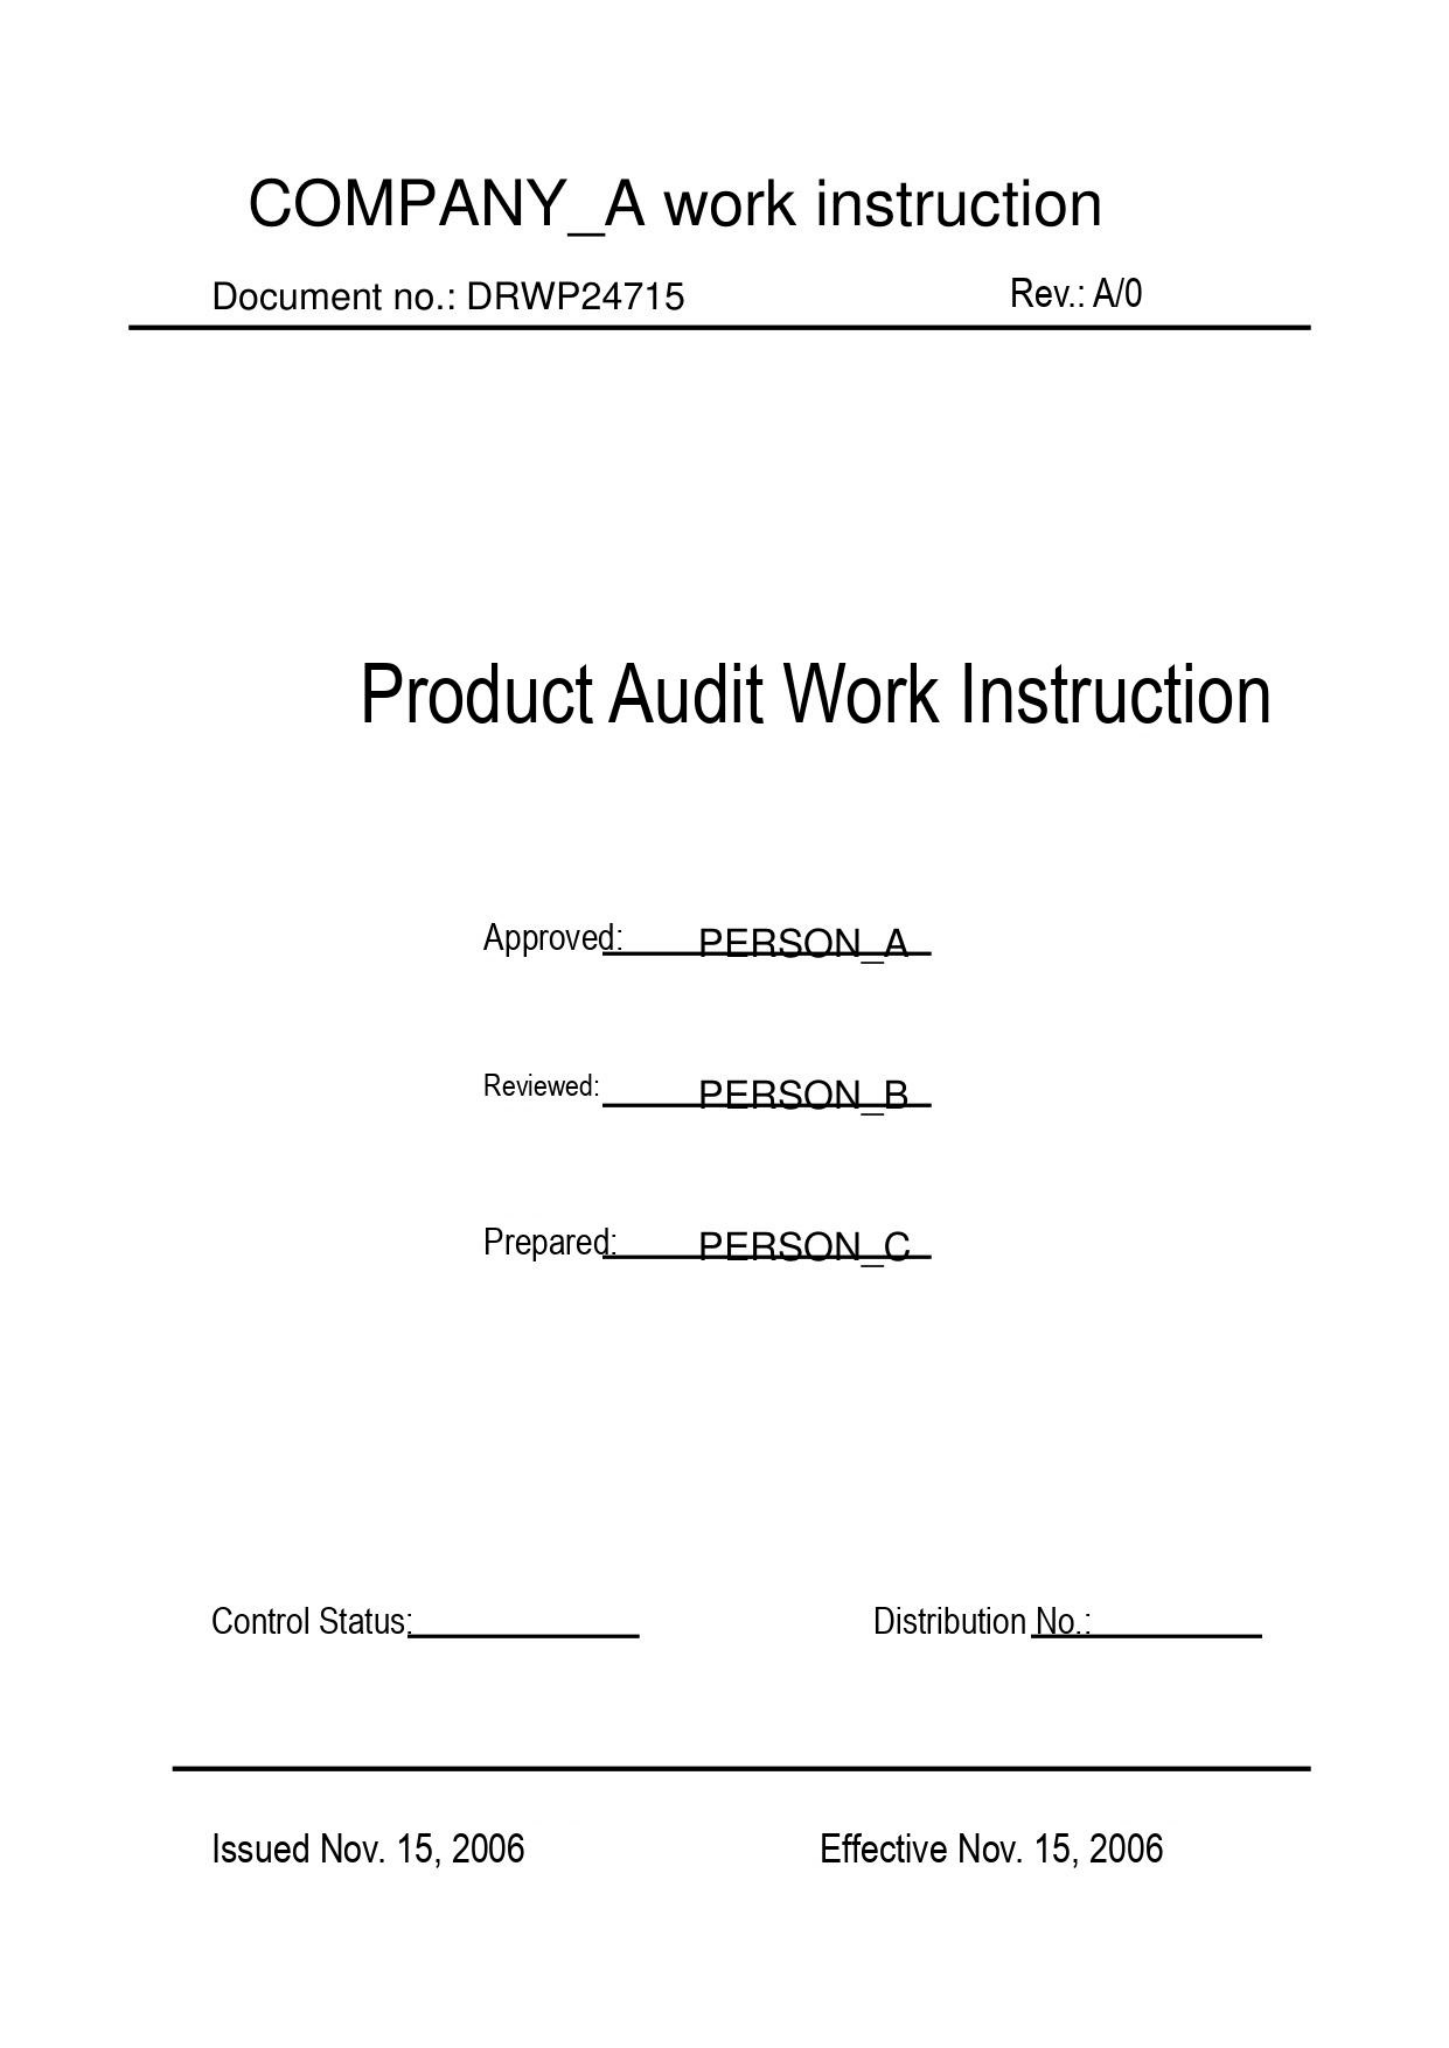COMPANY_A work instruction

Document no.: DRWP24715 Rev.: A/0

Product Audit Work Instruction

Approved: PERSON_A

Reviewed: PERSON_B

Prepared: PERSON_C

Control Status:

Distribution No.:

Issued Nov. 15, 2006 Effective Nov. 15, 2006
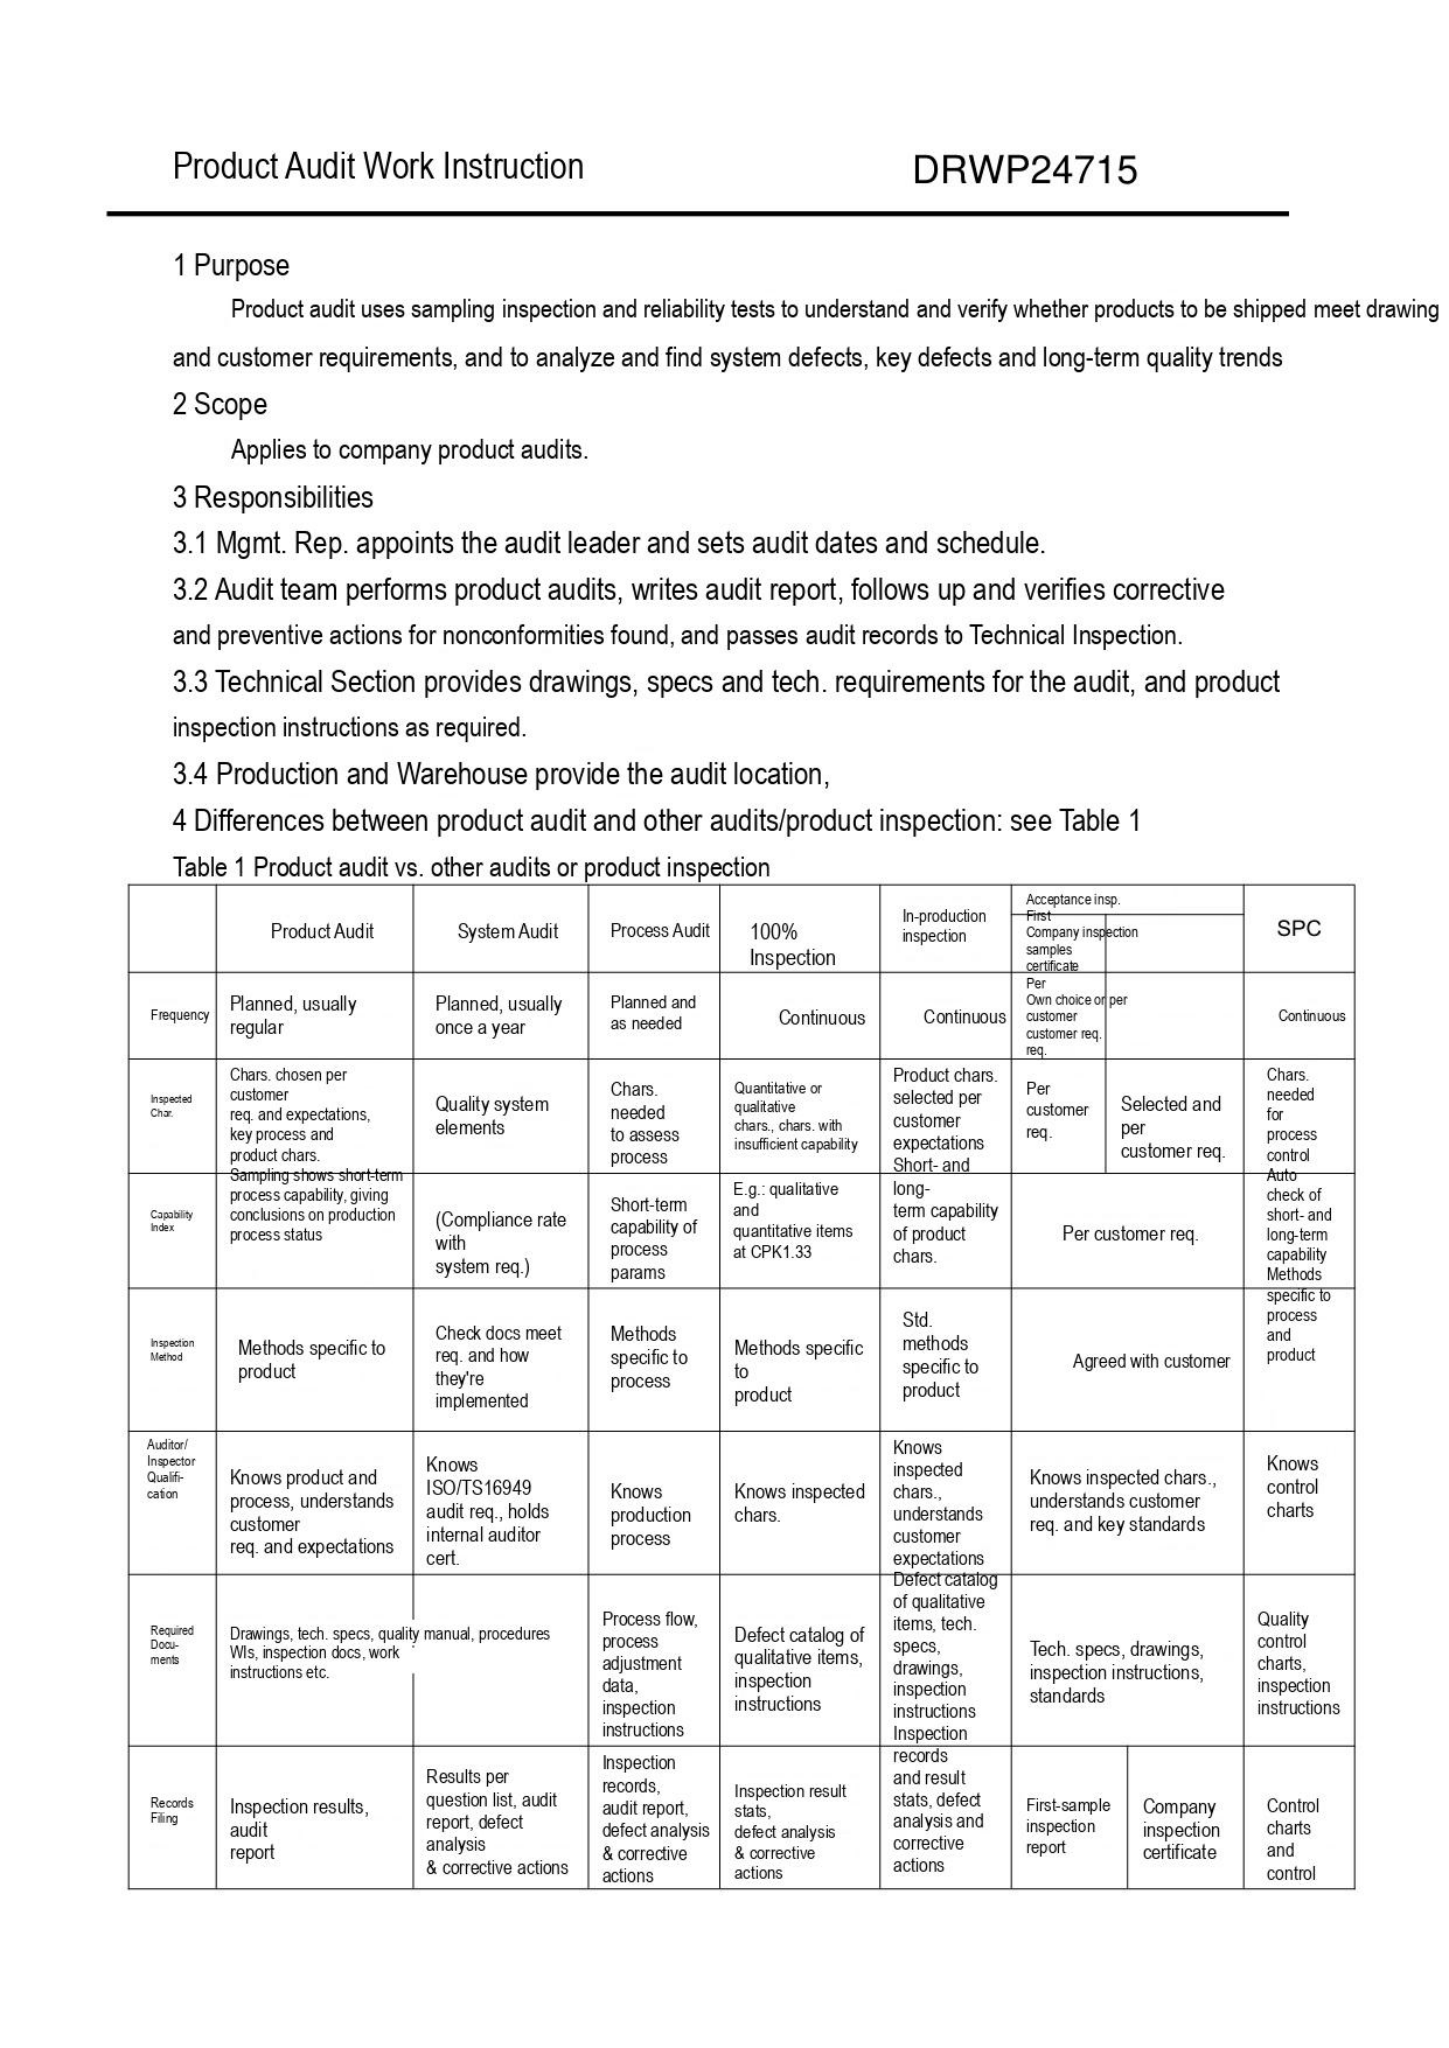Product Audit Work Instruction DRWP24715

1 Purpose

Product audit uses sampling inspection and reliability tests to understand and verify whether products to be shipped meet drawing and customer requirements, and to analyze and find system defects, key defects and long-term quality trends

2 Scope

Applies to company product audits.

3 Responsibilities

3.1 Mgmt. Rep. appoints the audit leader and sets audit dates and schedule.

3.2 Audit team performs product audits, writes audit report, follows up and verifies corrective and preventive actions for nonconformities found, and passes audit records to Technical Inspection.

3.3 Technical Section provides drawings, specs and tech. requirements for the audit, and product inspection instructions as required.

3.4 Production and Warehouse provide the audit location,

4 Differences between product audit and other audits/product inspection: see Table 1

Table 1 Product audit vs. other audits or product inspection

| | Product Audit | System Audit | Process Audit | 100% Inspection | In-production inspection | Acceptance insp. First samples | Acceptance insp. Company inspection certificate | SPC |
|---|---|---|---|---|---|---|---|---|
| Frequency | Planned, usually regular | Planned, usually once a year | Planned and as needed | Continuous | Continuous | Per customer customer req. | Own choice or per customer req. | Continuous |
| Inspected Char. | Chars. chosen per customer req. and expectations, key process and product chars. | Quality system elements | Chars. needed to assess process | Quantitative or qualitative chars., chars. with insufficient capability | Product chars. selected per customer expectations | Per customer req. | Selected and per customer req. | Chars. needed for process control |
| Capability Index | Sampling shows short-term process capability, giving conclusions on production process status | (Compliance rate with system req.) | Short-term capability of process params | E.g.: qualitative and quantitative items at CPK1.33 | Short- and long-term capability of product chars. | Per customer req. | Per customer req. | Auto check of short- and long-term capability |
| Inspection Method | Methods specific to product | Check docs meet req. and how they're implemented | Methods specific to process | Methods specific to product | Std. methods specific to product | Agreed with customer | Agreed with customer | Methods specific to process and product |
| Auditor/ Inspector Qualifi-cation | Knows product and process, understands customer req. and expectations | Knows ISO/TS16949 audit req., holds internal auditor cert. | Knows production process | Knows inspected chars. | Knows inspected chars., understands customer expectations | Knows inspected chars., understands customer req. and key standards | Knows inspected chars., understands customer req. and key standards | Knows control charts |
| Required Docu-ments | Drawings, tech. specs, quality WIs, inspection docs, work instructions etc. | manual, procedures | Process flow, process adjustment data, inspection instructions | Defect catalog of qualitative items, inspection instructions | Defect catalog of qualitative items, tech. specs, drawings, inspection instructions | Tech. specs, drawings, inspection instructions, standards | Tech. specs, drawings, inspection instructions, standards | Quality control charts, inspection instructions |
| Records Filing | Inspection results, audit report | Results per question list, audit report, defect analysis & corrective actions | Inspection records, audit report, defect analysis & corrective actions | Inspection result stats, defect analysis & corrective actions | Inspection records and result stats, defect analysis and corrective actions | First-sample inspection report | Company inspection certificate | Control charts and control |
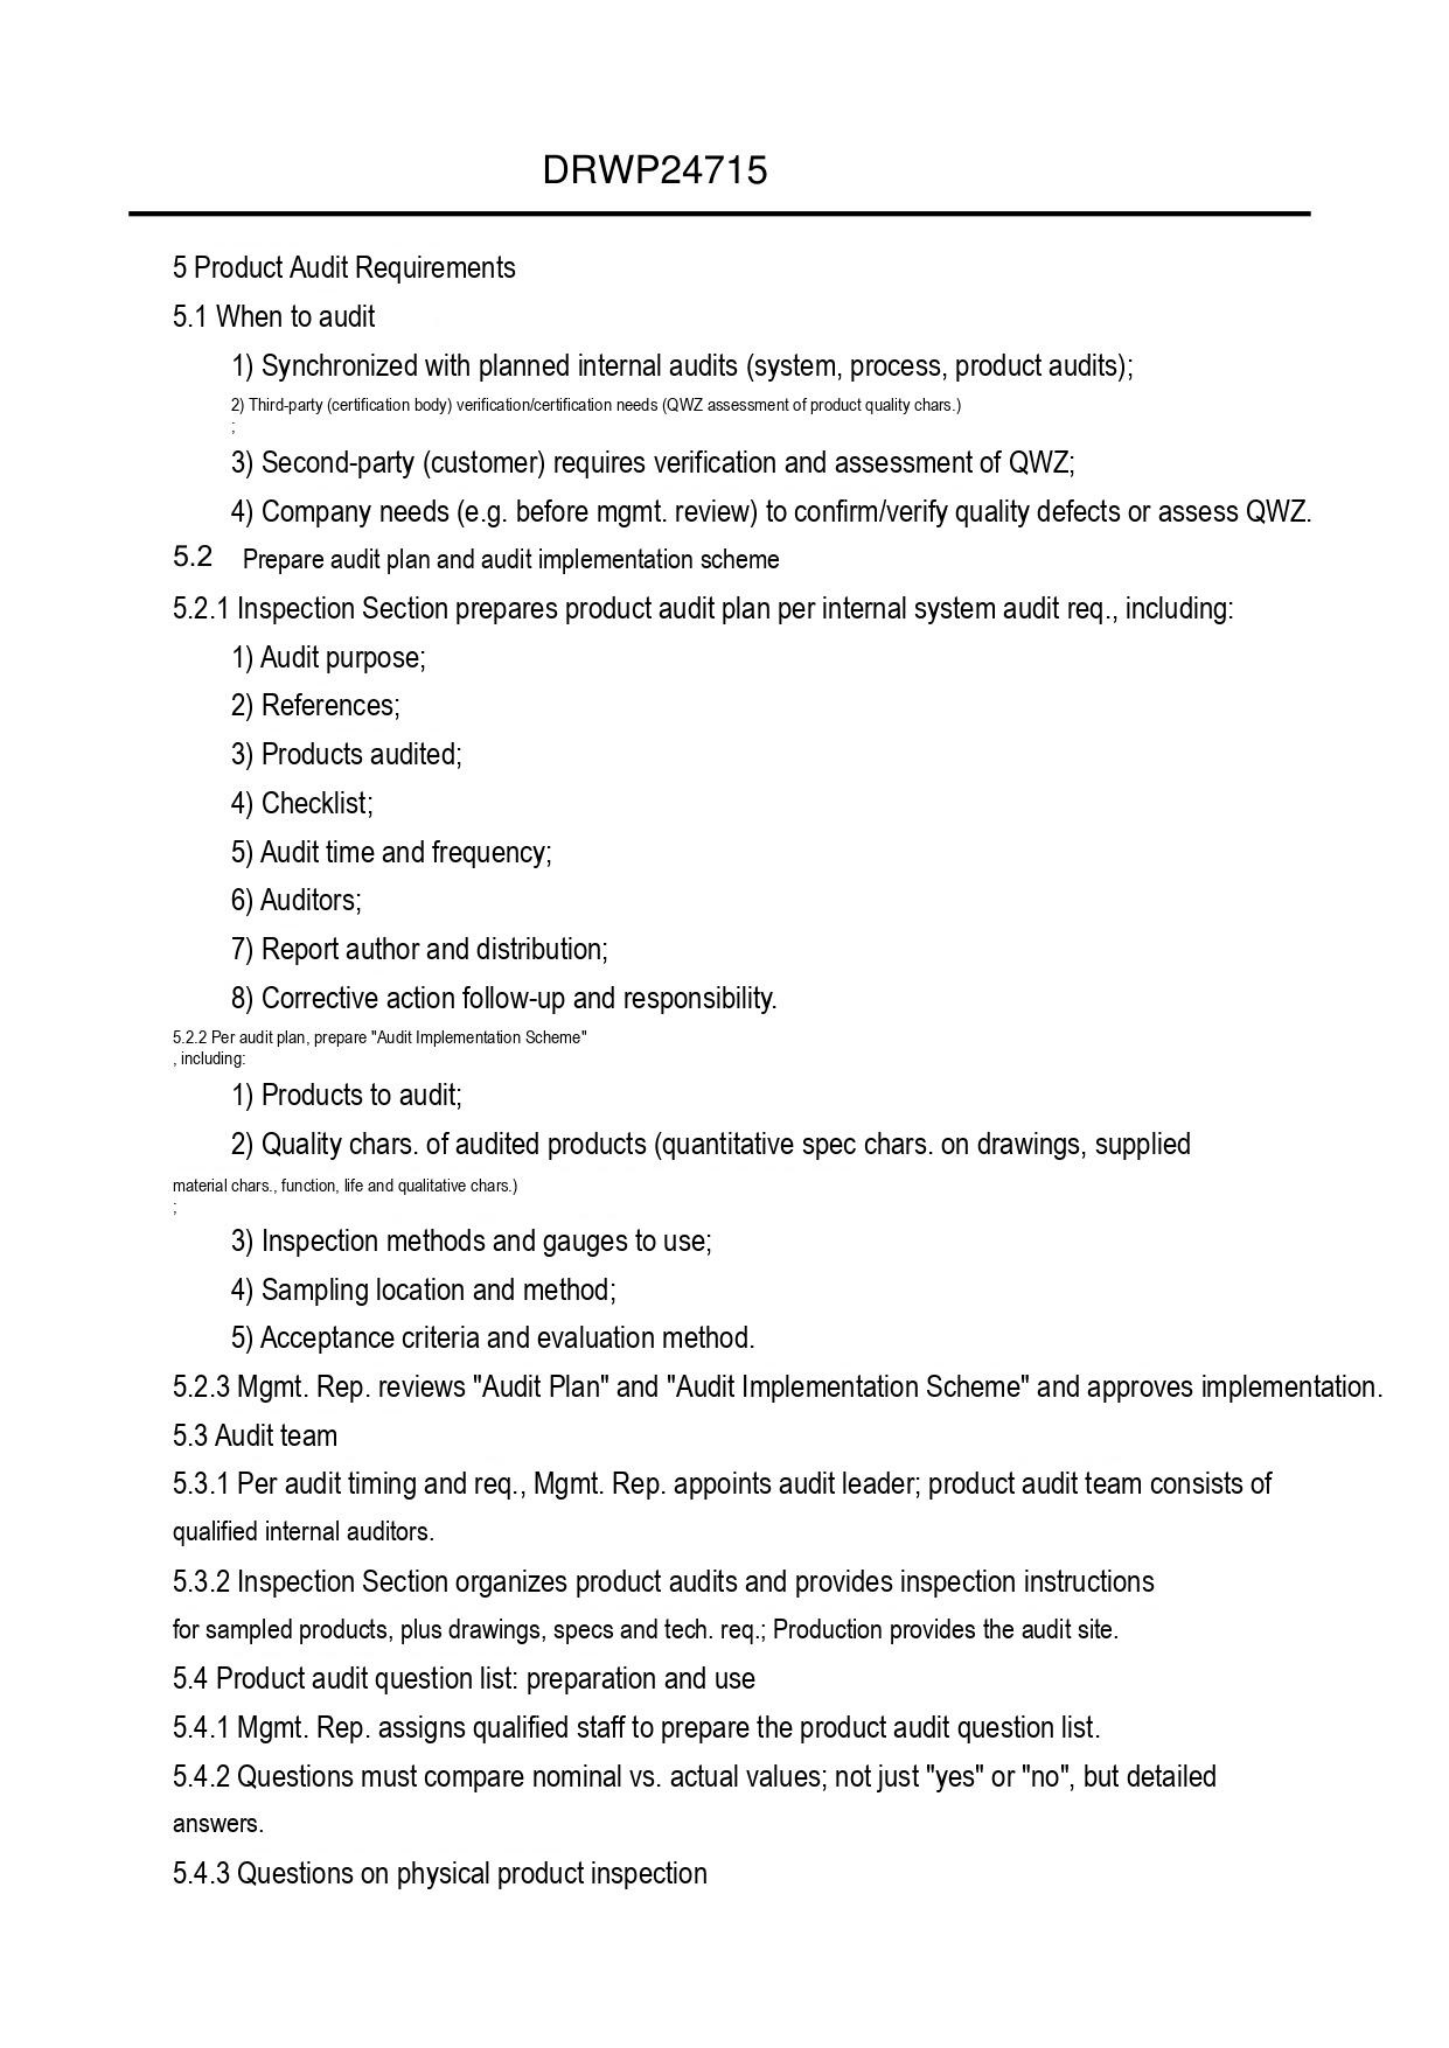DRWP24715

5 Product Audit Requirements

5.1 When to audit

1) Synchronized with planned internal audits (system, process, product audits);

2) Third-party (certification body) verification/certification needs (QWZ assessment of product quality chars.)
;

3) Second-party (customer) requires verification and assessment of QWZ;

4) Company needs (e.g. before mgmt. review) to confirm/verify quality defects or assess QWZ.

5.2 Prepare audit plan and audit implementation scheme

5.2.1 Inspection Section prepares product audit plan per internal system audit req., including:

1) Audit purpose;

2) References;

3) Products audited;

4) Checklist;

5) Audit time and frequency;

6) Auditors;

7) Report author and distribution;

8) Corrective action follow-up and responsibility.

5.2.2 Per audit plan, prepare "Audit Implementation Scheme"
, including:

1) Products to audit;

2) Quality chars. of audited products (quantitative spec chars. on drawings, supplied material chars., function, life and qualitative chars.)
;

3) Inspection methods and gauges to use;

4) Sampling location and method;

5) Acceptance criteria and evaluation method.

5.2.3 Mgmt. Rep. reviews "Audit Plan" and "Audit Implementation Scheme" and approves implementation.

5.3 Audit team

5.3.1 Per audit timing and req., Mgmt. Rep. appoints audit leader; product audit team consists of qualified internal auditors.

5.3.2 Inspection Section organizes product audits and provides inspection instructions for sampled products, plus drawings, specs and tech. req.; Production provides the audit site.

5.4 Product audit question list: preparation and use

5.4.1 Mgmt. Rep. assigns qualified staff to prepare the product audit question list.

5.4.2 Questions must compare nominal vs. actual values; not just "yes" or "no", but detailed answers.

5.4.3 Questions on physical product inspection
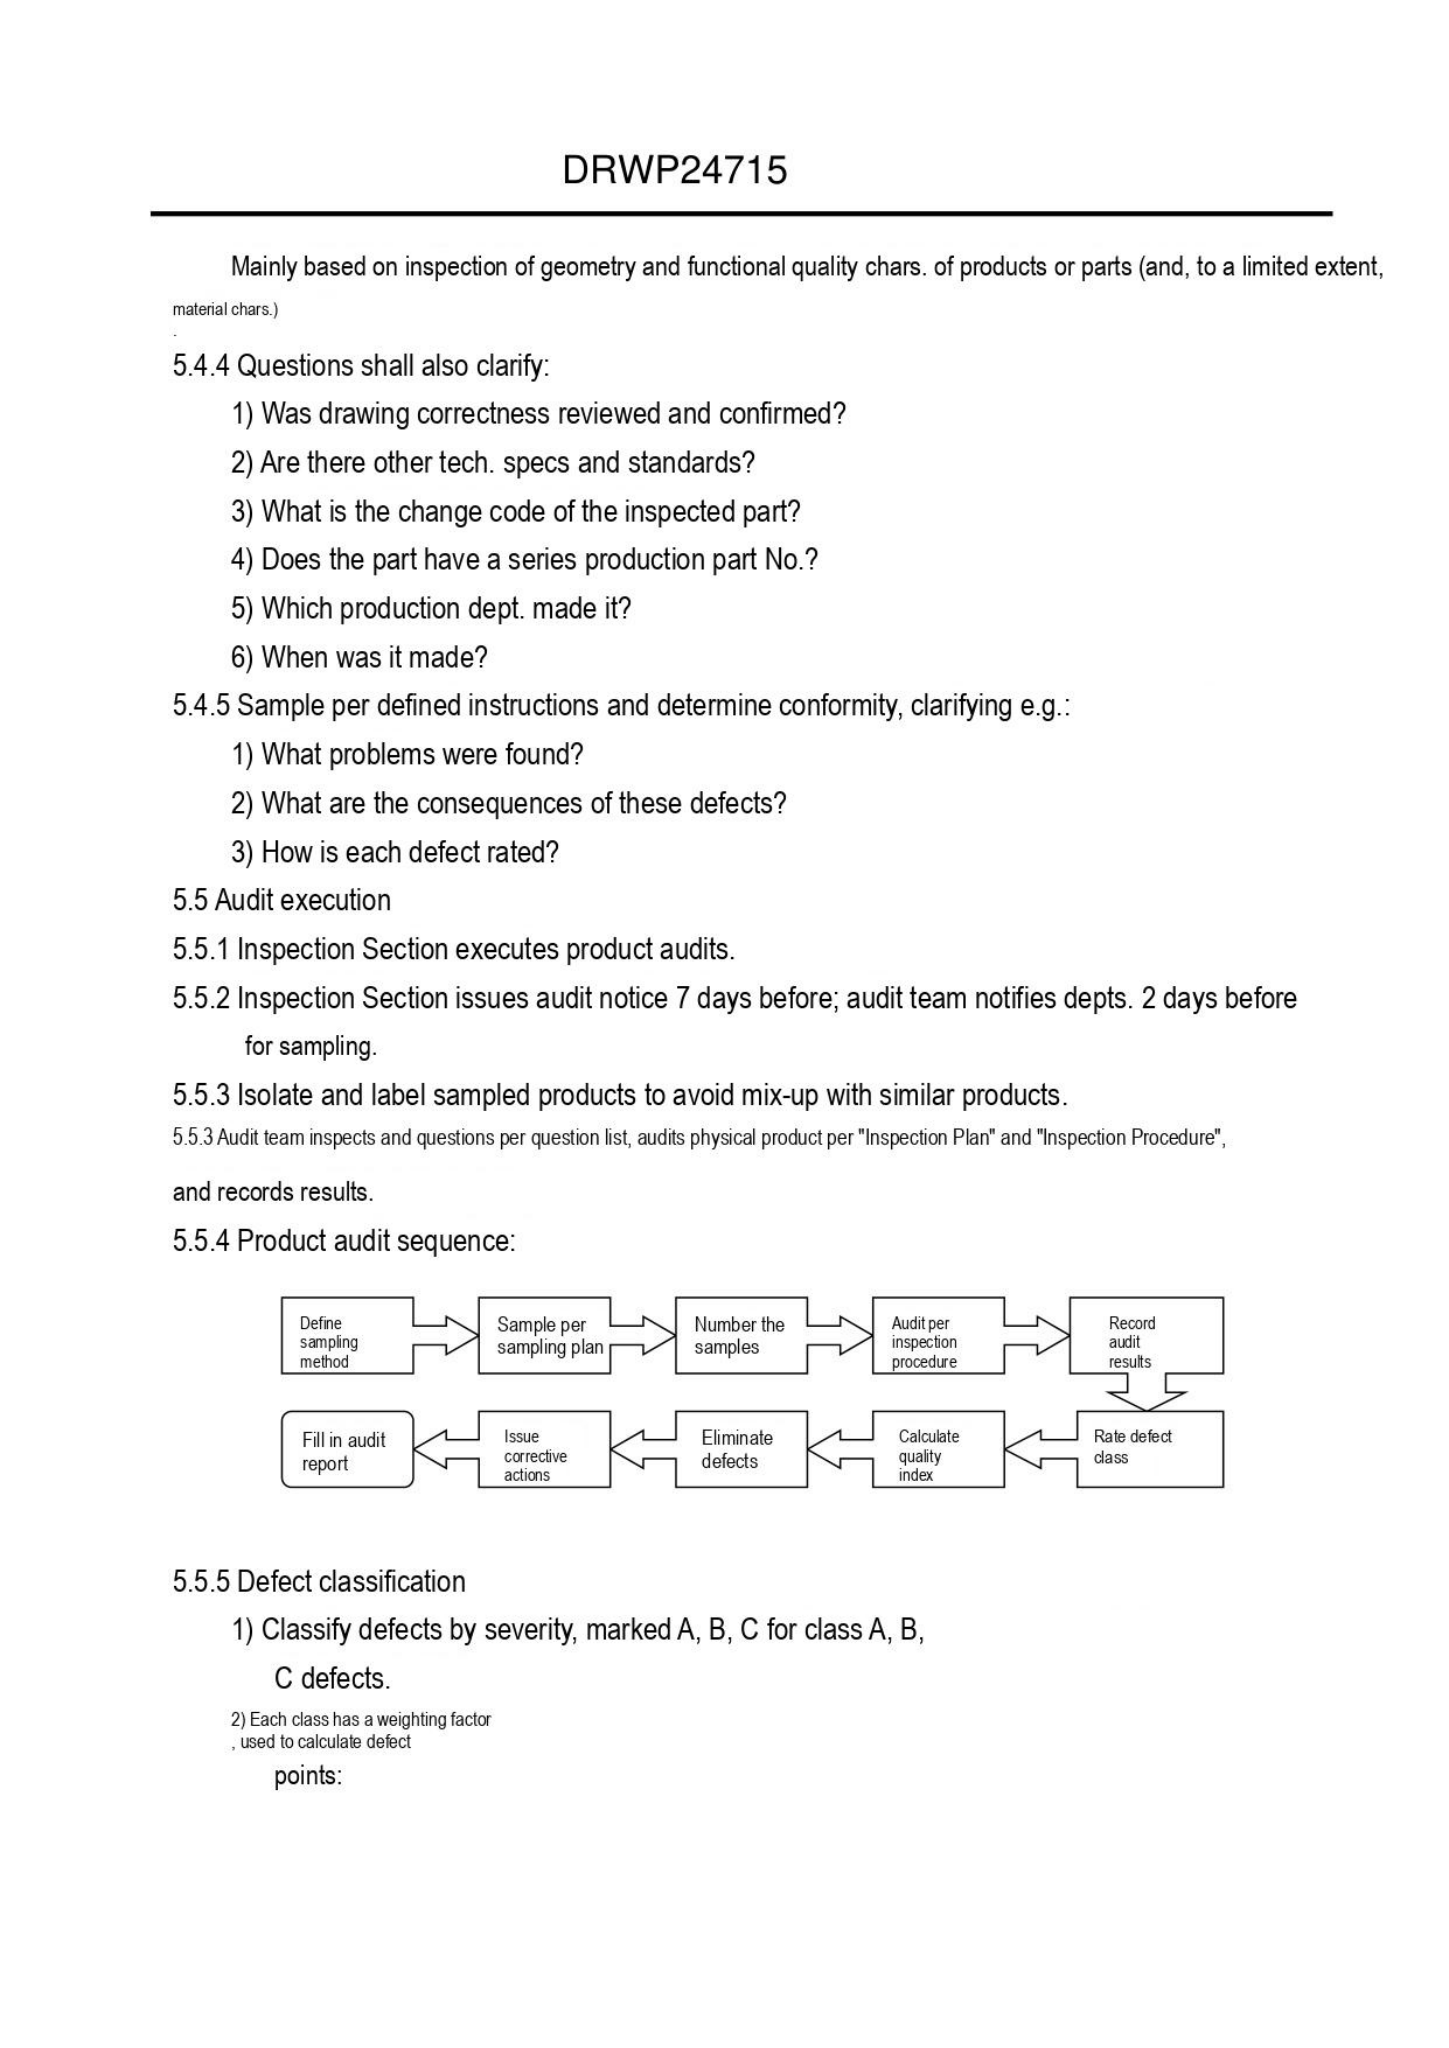DRWP24715

Mainly based on inspection of geometry and functional quality chars. of products or parts (and, to a limited extent, material chars.)

5.4.4 Questions shall also clarify:

1) Was drawing correctness reviewed and confirmed?

2) Are there other tech. specs and standards?

3) What is the change code of the inspected part?

4) Does the part have a series production part No.?

5) Which production dept. made it?

6) When was it made?

5.4.5 Sample per defined instructions and determine conformity, clarifying e.g.:

1) What problems were found?

2) What are the consequences of these defects?

3) How is each defect rated?

5.5 Audit execution

5.5.1 Inspection Section executes product audits.

5.5.2 Inspection Section issues audit notice 7 days before; audit team notifies depts. 2 days before for sampling.

5.5.3 Isolate and label sampled products to avoid mix-up with similar products.

5.5.3 Audit team inspects and questions per question list, audits physical product per "Inspection Plan" and "Inspection Procedure", and records results.

5.5.4 Product audit sequence:

Define sampling method → Sample per sampling plan → Number the samples → Audit per inspection procedure → Record audit results → Rate defect class → Calculate quality index → Eliminate defects → Issue corrective actions → Fill in audit report

5.5.5 Defect classification

1) Classify defects by severity, marked A, B, C for class A, B, C defects.

2) Each class has a weighting factor, used to calculate defect points:
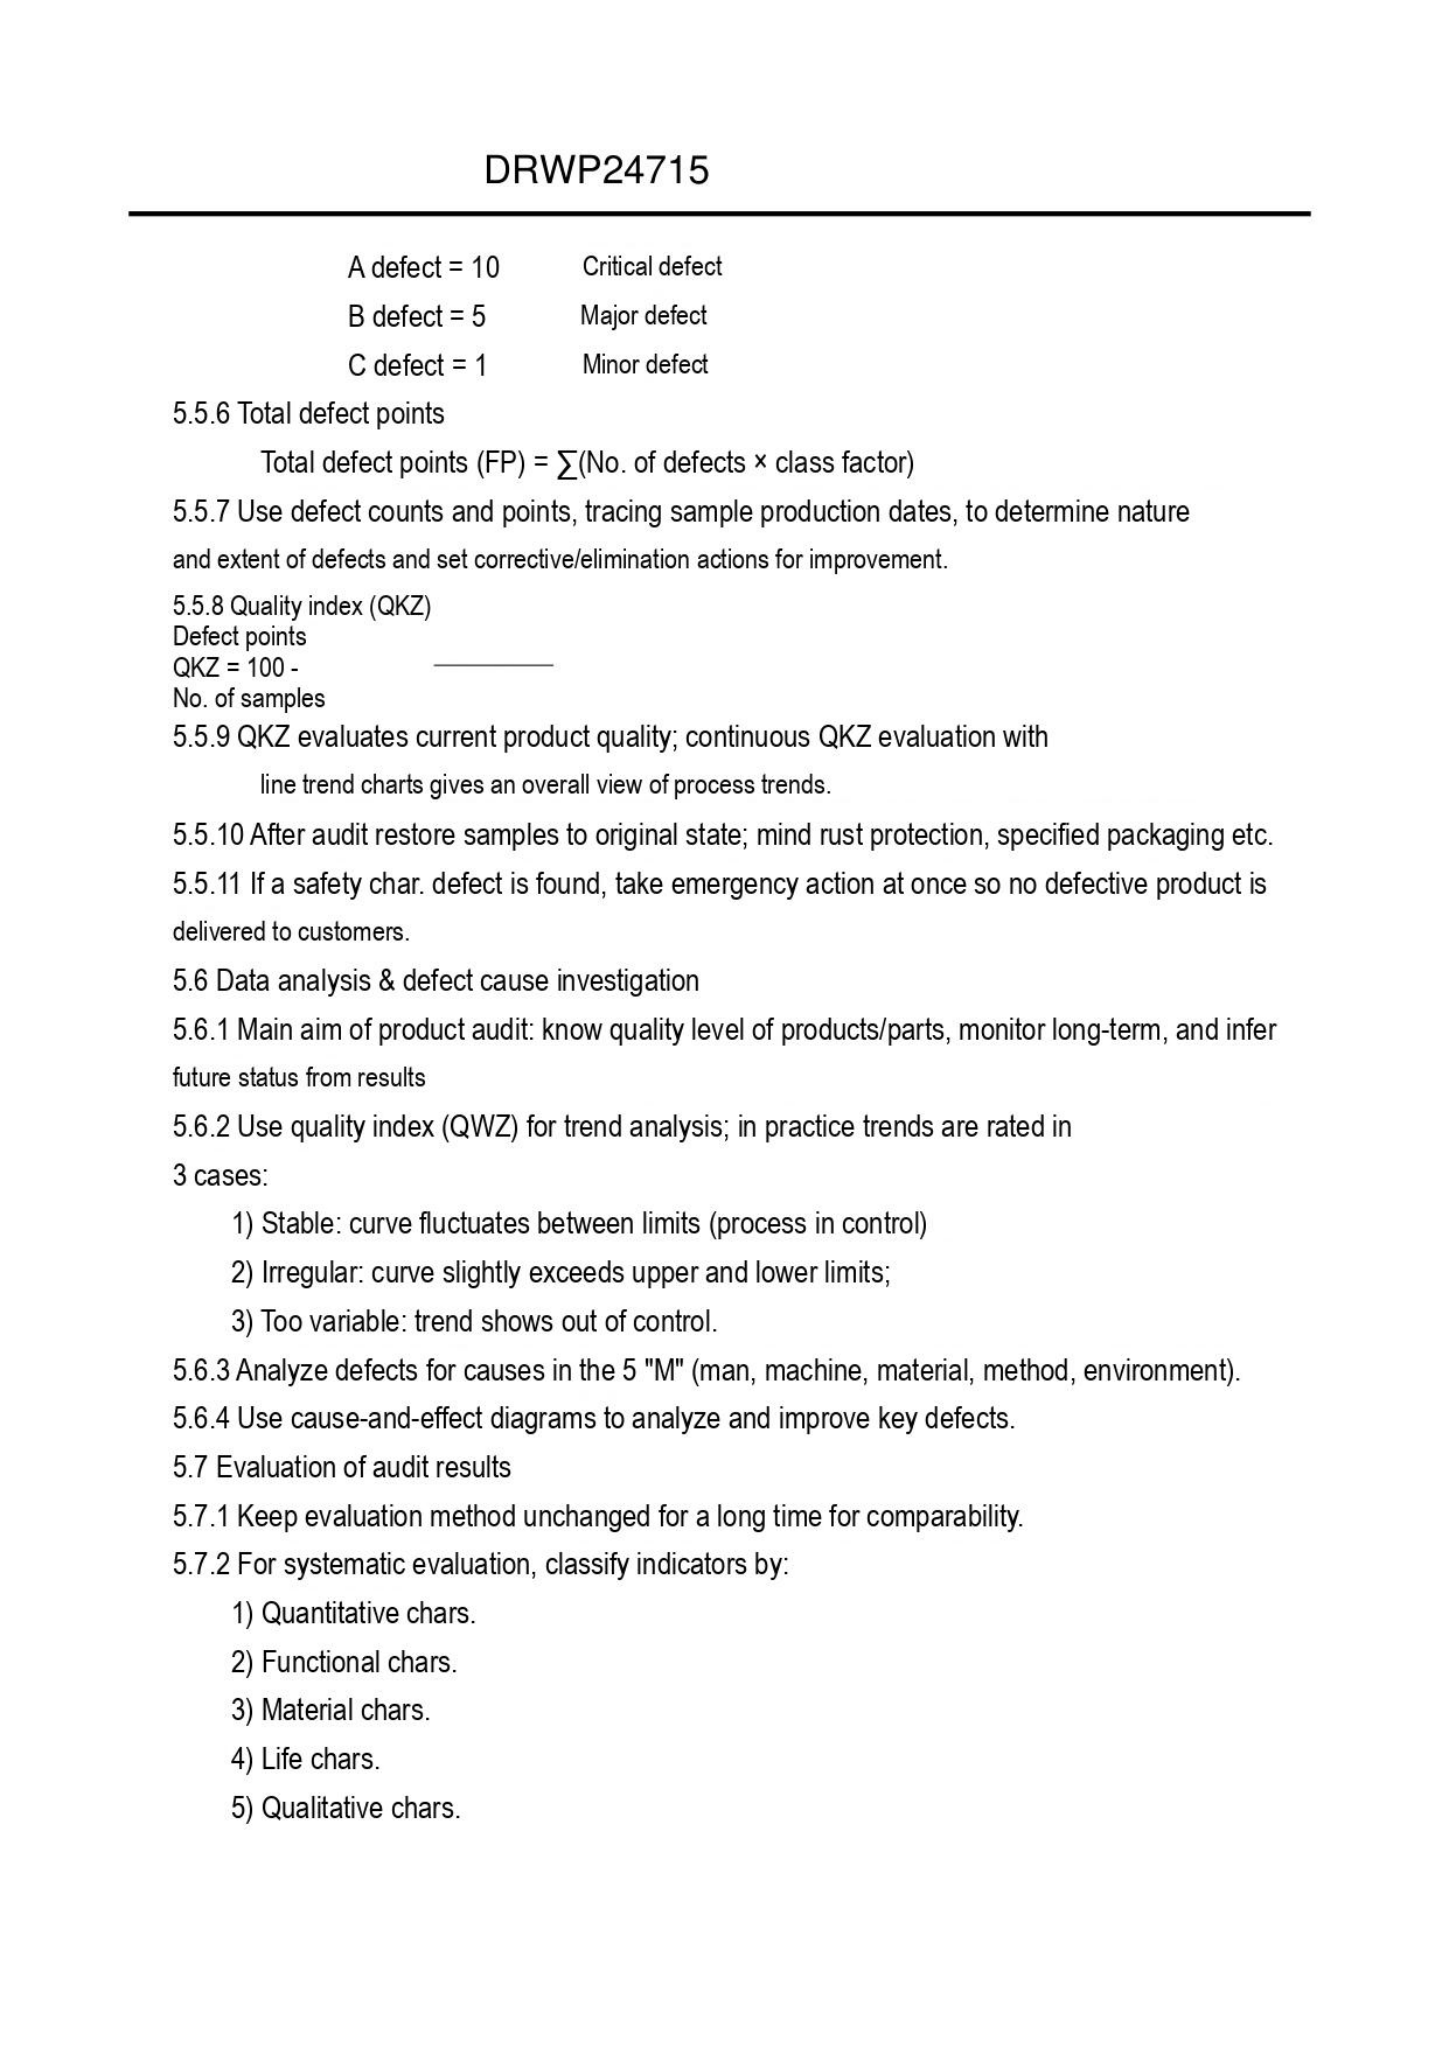DRWP24715

A defect = 10 Critical defect
B defect = 5 Major defect
C defect = 1 Minor defect

5.5.6 Total defect points

Total defect points (FP) = ∑(No. of defects × class factor)

5.5.7 Use defect counts and points, tracing sample production dates, to determine nature and extent of defects and set corrective/elimination actions for improvement.

5.5.8 Quality index (QKZ)
Defect points
QKZ = 100 -
No. of samples

5.5.9 QKZ evaluates current product quality; continuous QKZ evaluation with line trend charts gives an overall view of process trends.

5.5.10 After audit restore samples to original state; mind rust protection, specified packaging etc.

5.5.11 If a safety char. defect is found, take emergency action at once so no defective product is delivered to customers.

5.6 Data analysis & defect cause investigation

5.6.1 Main aim of product audit: know quality level of products/parts, monitor long-term, and infer future status from results

5.6.2 Use quality index (QWZ) for trend analysis; in practice trends are rated in 3 cases:

1) Stable: curve fluctuates between limits (process in control)
2) Irregular: curve slightly exceeds upper and lower limits;
3) Too variable: trend shows out of control.

5.6.3 Analyze defects for causes in the 5 "M" (man, machine, material, method, environment).

5.6.4 Use cause-and-effect diagrams to analyze and improve key defects.

5.7 Evaluation of audit results

5.7.1 Keep evaluation method unchanged for a long time for comparability.

5.7.2 For systematic evaluation, classify indicators by:

1) Quantitative chars.
2) Functional chars.
3) Material chars.
4) Life chars.
5) Qualitative chars.
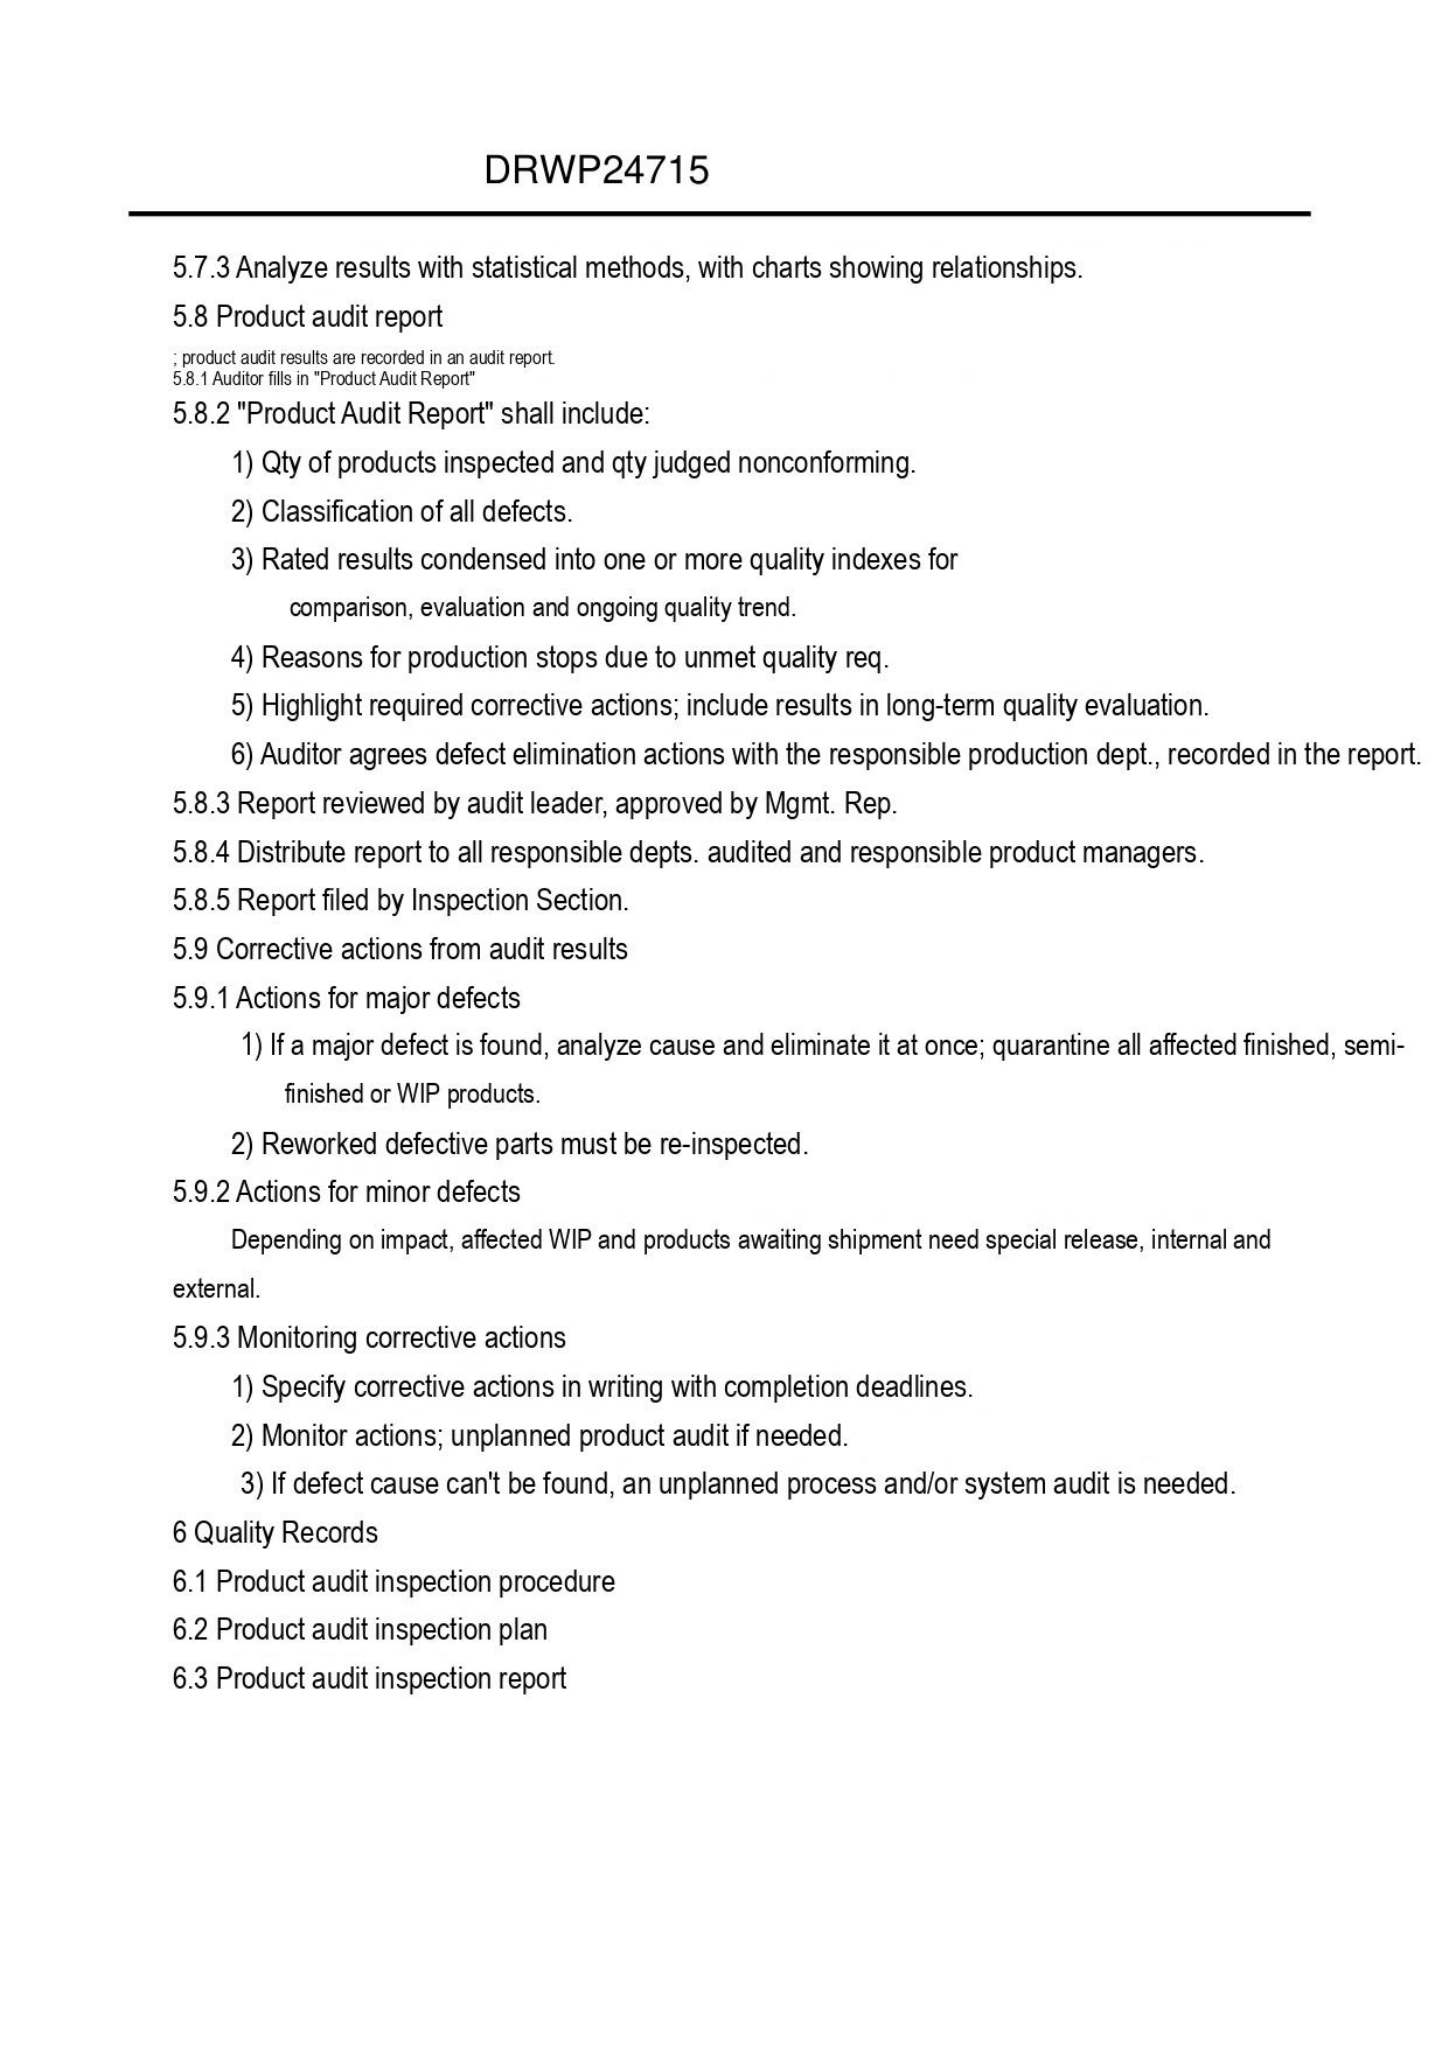DRWP24715

5.7.3 Analyze results with statistical methods, with charts showing relationships.

5.8 Product audit report

; product audit results are recorded in an audit report.
5.8.1 Auditor fills in "Product Audit Report"

5.8.2 "Product Audit Report" shall include:

1) Qty of products inspected and qty judged nonconforming.

2) Classification of all defects.

3) Rated results condensed into one or more quality indexes for comparison, evaluation and ongoing quality trend.

4) Reasons for production stops due to unmet quality req.

5) Highlight required corrective actions; include results in long-term quality evaluation.

6) Auditor agrees defect elimination actions with the responsible production dept., recorded in the report.

5.8.3 Report reviewed by audit leader, approved by Mgmt. Rep.

5.8.4 Distribute report to all responsible depts. audited and responsible product managers.

5.8.5 Report filed by Inspection Section.

5.9 Corrective actions from audit results

5.9.1 Actions for major defects

1) If a major defect is found, analyze cause and eliminate it at once; quarantine all affected finished, semi-finished or WIP products.

2) Reworked defective parts must be re-inspected.

5.9.2 Actions for minor defects

Depending on impact, affected WIP and products awaiting shipment need special release, internal and external.

5.9.3 Monitoring corrective actions

1) Specify corrective actions in writing with completion deadlines.

2) Monitor actions; unplanned product audit if needed.

3) If defect cause can't be found, an unplanned process and/or system audit is needed.

6 Quality Records

6.1 Product audit inspection procedure

6.2 Product audit inspection plan

6.3 Product audit inspection report
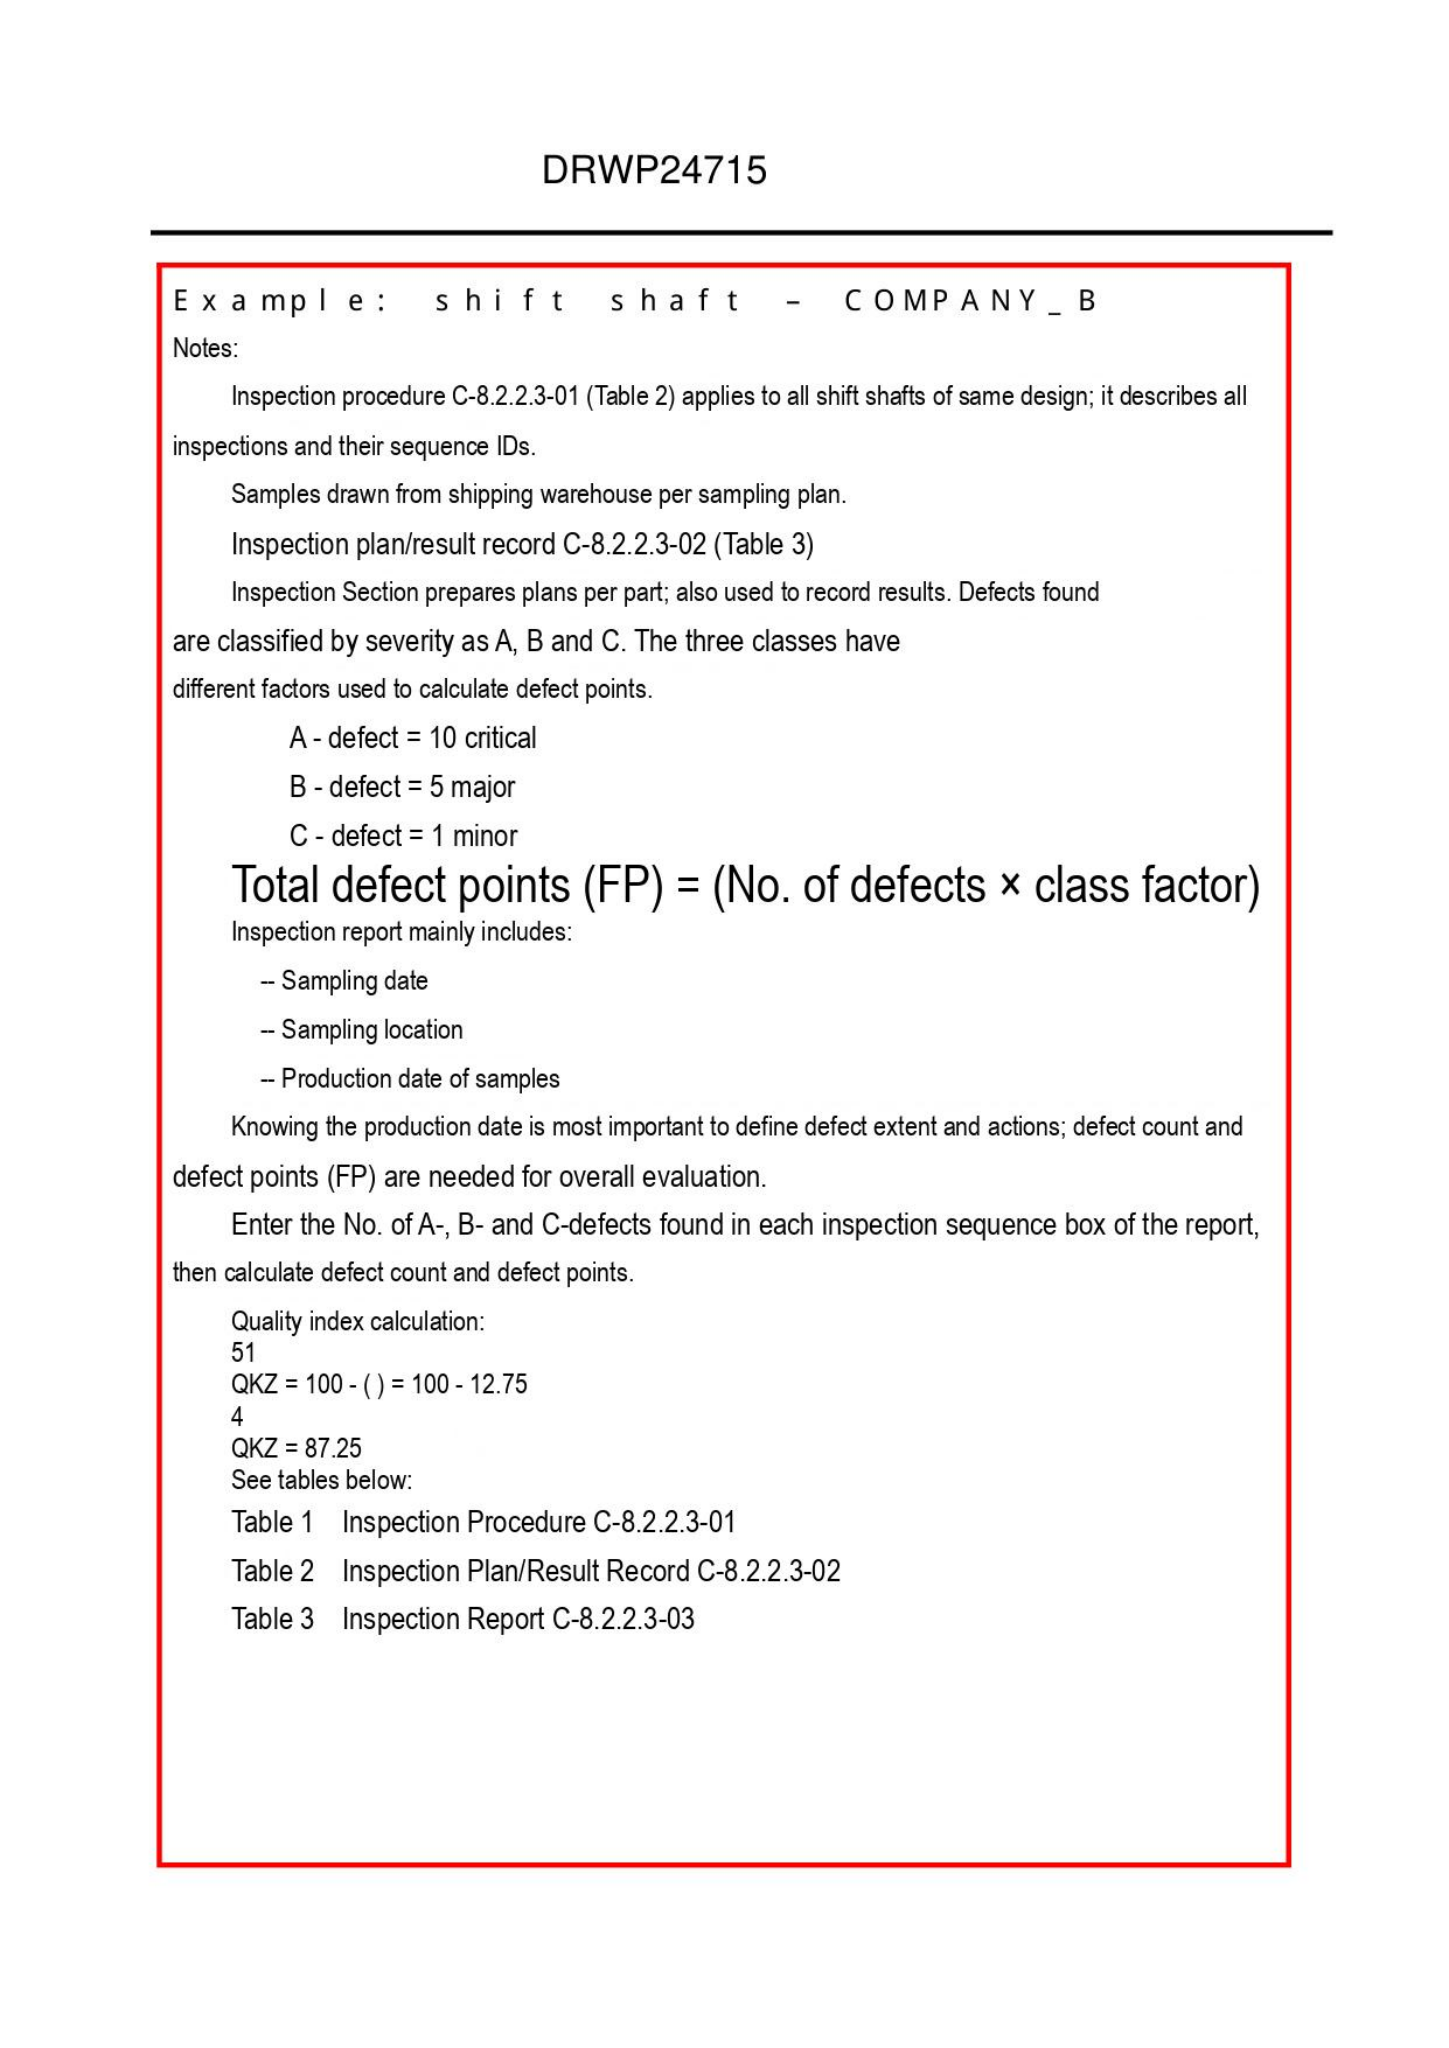DRWP24715

Example: shift shaft – COMPANY_B

Notes:

Inspection procedure C-8.2.2.3-01 (Table 2) applies to all shift shafts of same design; it describes all inspections and their sequence IDs.

Samples drawn from shipping warehouse per sampling plan.

Inspection plan/result record C-8.2.2.3-02 (Table 3)

Inspection Section prepares plans per part; also used to record results. Defects found are classified by severity as A, B and C. The three classes have different factors used to calculate defect points.

A - defect = 10 critical

B - defect = 5 major

C - defect = 1 minor

Total defect points (FP) = (No. of defects × class factor)

Inspection report mainly includes:

-- Sampling date

-- Sampling location

-- Production date of samples

Knowing the production date is most important to define defect extent and actions; defect count and defect points (FP) are needed for overall evaluation.

Enter the No. of A-, B- and C-defects found in each inspection sequence box of the report, then calculate defect count and defect points.

Quality index calculation:
51
QKZ = 100 - ( ) = 100 - 12.75
4
QKZ = 87.25
See tables below:

Table 1 Inspection Procedure C-8.2.2.3-01

Table 2 Inspection Plan/Result Record C-8.2.2.3-02

Table 3 Inspection Report C-8.2.2.3-03